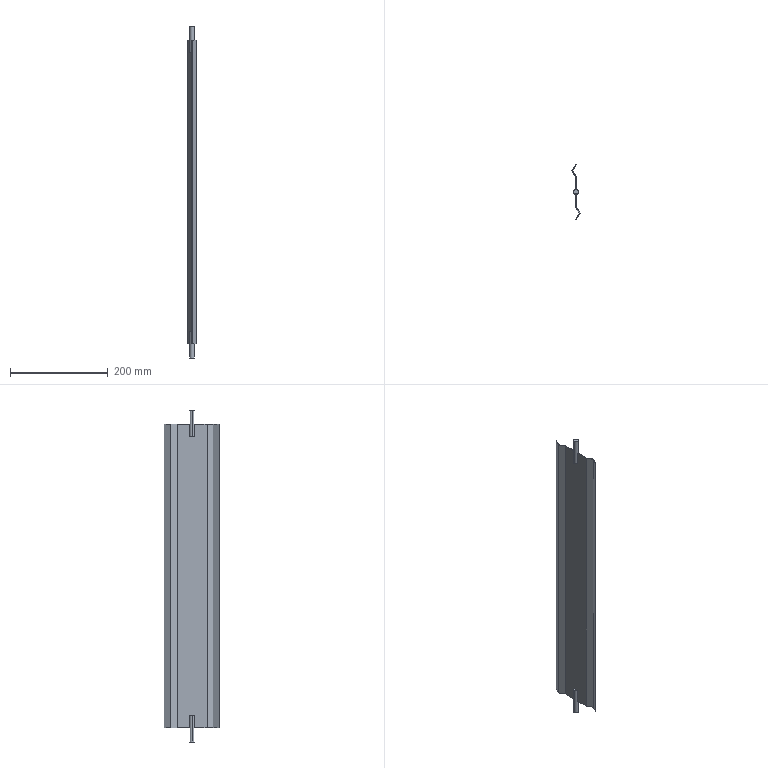Part | SolidWorks | features Extrusion 1, ICE 1, MirrorPattern 1 | 1 solid | 26 faces | box 16.5 x 113 x 678 mm | volume 119565 mm3 | plane 22 | cylinder 4 | commonest cylinder face diameters 10 x4
STEP:
#1=CARTESIAN_POINT('',(4.25,56.5,-284.));
#2=VERTEX_POINT('',#1);
#3=CARTESIAN_POINT('',(0.,61.443,-284.));
#4=VERTEX_POINT('',#3);
#5=CARTESIAN_POINT('',(-0.75,56.5,-284.));
#6=DIRECTION('',(0.,0.,1.));
#7=DIRECTION('',(1.,0.,0.));
#8=AXIS2_PLACEMENT_3D('',#5,#6,#7);
#9=CIRCLE('',#8,5.);
#10=EDGE_CURVE('',#2,#4,#9,.T.);
#11=ORIENTED_EDGE('',*,*,#10,.F.);
#12=CARTESIAN_POINT('',(4.25,56.5,-339.));
#13=VERTEX_POINT('',#12);
#14=CARTESIAN_POINT('',(4.25,56.5,-284.));
#15=DIRECTION('',(0.,0.,-1.));
#16=VECTOR('',#15,1000.);
#17=LINE('',#14,#16);
#18=EDGE_CURVE('',#2,#13,#17,.T.);
#19=ORIENTED_EDGE('',*,*,#18,.T.);
#20=CARTESIAN_POINT('',(-5.75,56.5,-339.));
#21=VERTEX_POINT('',#20);
#22=CARTESIAN_POINT('',(-0.75,56.5,-339.));
#23=DIRECTION('',(0.,0.,1.));
#24=DIRECTION('',(1.,0.,0.));
#25=AXIS2_PLACEMENT_3D('',#22,#23,#24);
#26=CIRCLE('',#25,5.);
#27=EDGE_CURVE('',#13,#21,#26,.T.);
#28=ORIENTED_EDGE('',*,*,#27,.T.);
#29=CARTESIAN_POINT('',(-5.75,56.5,-284.));
#30=VERTEX_POINT('',#29);
#31=CARTESIAN_POINT('',(-5.75,56.5,-284.));
#32=DIRECTION('',(0.,0.,-1.));
#33=VECTOR('',#32,1000.);
#34=LINE('',#31,#33);
#35=EDGE_CURVE('',#30,#21,#34,.T.);
#36=ORIENTED_EDGE('',*,*,#35,.F.);
#37=CARTESIAN_POINT('',(-1.5,61.443,-284.));
#38=VERTEX_POINT('',#37);
#39=CARTESIAN_POINT('',(-0.75,56.5,-284.));
#40=DIRECTION('',(0.,0.,1.));
#41=DIRECTION('',(1.,0.,0.));
#42=AXIS2_PLACEMENT_3D('',#39,#40,#41);
#43=CIRCLE('',#42,5.);
#44=EDGE_CURVE('',#38,#30,#43,.T.);
#45=ORIENTED_EDGE('',*,*,#44,.F.);
#46=CARTESIAN_POINT('',(-1.5,61.443,-310.));
#47=VERTEX_POINT('',#46);
#48=CARTESIAN_POINT('',(-1.5,61.443,-284.));
#49=DIRECTION('',(0.,0.,-1.));
#50=VECTOR('',#49,1000.);
#51=LINE('',#48,#50);
#52=EDGE_CURVE('',#38,#47,#51,.T.);
#53=ORIENTED_EDGE('',*,*,#52,.T.);
#54=CARTESIAN_POINT('',(0.,61.443,-310.));
#55=VERTEX_POINT('',#54);
#56=CARTESIAN_POINT('',(-0.75,56.5,-310.));
#57=DIRECTION('',(0.,0.,1.));
#58=DIRECTION('',(-1.,0.,0.));
#59=AXIS2_PLACEMENT_3D('',#56,#57,#58);
#60=CIRCLE('',#59,5.);
#61=EDGE_CURVE('',#55,#47,#60,.T.);
#62=ORIENTED_EDGE('',*,*,#61,.F.);
#63=CARTESIAN_POINT('',(0.,61.443,-284.));
#64=DIRECTION('',(0.,0.,1.));
#65=VECTOR('',#64,1000.);
#66=LINE('',#63,#65);
#67=EDGE_CURVE('',#55,#4,#66,.T.);
#68=ORIENTED_EDGE('',*,*,#67,.T.);
#69=EDGE_LOOP('',(#11,#19,#28,#36,#45,#53,#62,#68));
#70=FACE_OUTER_BOUND('',#69,.T.);
#71=CARTESIAN_POINT('',(-0.75,56.5,-284.));
#72=DIRECTION('',(0.,0.,-1.));
#73=DIRECTION('',(-1.,0.,0.));
#74=AXIS2_PLACEMENT_3D('',#71,#72,#73);
#75=CYLINDRICAL_SURFACE('',#74,5.);
#76=ADVANCED_FACE('',(#70),#75,.T.);
#77=CARTESIAN_POINT('',(-1.5,61.443,284.));
#78=VERTEX_POINT('',#77);
#79=CARTESIAN_POINT('',(-5.75,56.5,284.));
#80=VERTEX_POINT('',#79);
#81=CARTESIAN_POINT('',(-0.75,56.5,284.));
#82=DIRECTION('',(0.,0.,1.));
#83=DIRECTION('',(1.,0.,0.));
#84=AXIS2_PLACEMENT_3D('',#81,#82,#83);
#85=CIRCLE('',#84,5.);
#86=EDGE_CURVE('',#78,#80,#85,.T.);
#87=ORIENTED_EDGE('',*,*,#86,.T.);
#88=CARTESIAN_POINT('',(-5.75,56.5,339.));
#89=VERTEX_POINT('',#88);
#90=CARTESIAN_POINT('',(-5.75,56.5,284.));
#91=DIRECTION('',(0.,0.,1.));
#92=VECTOR('',#91,1000.);
#93=LINE('',#90,#92);
#94=EDGE_CURVE('',#80,#89,#93,.T.);
#95=ORIENTED_EDGE('',*,*,#94,.T.);
#96=CARTESIAN_POINT('',(4.25,56.5,339.));
#97=VERTEX_POINT('',#96);
#98=CARTESIAN_POINT('',(-0.75,56.5,339.));
#99=DIRECTION('',(0.,0.,1.));
#100=DIRECTION('',(1.,0.,0.));
#101=AXIS2_PLACEMENT_3D('',#98,#99,#100);
#102=CIRCLE('',#101,5.);
#103=EDGE_CURVE('',#97,#89,#102,.T.);
#104=ORIENTED_EDGE('',*,*,#103,.F.);
#105=CARTESIAN_POINT('',(4.25,56.5,284.));
#106=VERTEX_POINT('',#105);
#107=CARTESIAN_POINT('',(4.25,56.5,284.));
#108=DIRECTION('',(0.,0.,1.));
#109=VECTOR('',#108,1000.);
#110=LINE('',#107,#109);
#111=EDGE_CURVE('',#106,#97,#110,.T.);
#112=ORIENTED_EDGE('',*,*,#111,.F.);
#113=CARTESIAN_POINT('',(0.,61.443,284.));
#114=VERTEX_POINT('',#113);
#115=CARTESIAN_POINT('',(-0.75,56.5,284.));
#116=DIRECTION('',(0.,0.,1.));
#117=DIRECTION('',(1.,0.,0.));
#118=AXIS2_PLACEMENT_3D('',#115,#116,#117);
#119=CIRCLE('',#118,5.);
#120=EDGE_CURVE('',#106,#114,#119,.T.);
#121=ORIENTED_EDGE('',*,*,#120,.T.);
#122=CARTESIAN_POINT('',(0.,61.443,310.));
#123=VERTEX_POINT('',#122);
#124=CARTESIAN_POINT('',(0.,61.443,284.));
#125=DIRECTION('',(0.,0.,-1.));
#126=VECTOR('',#125,1000.);
#127=LINE('',#124,#126);
#128=EDGE_CURVE('',#123,#114,#127,.T.);
#129=ORIENTED_EDGE('',*,*,#128,.F.);
#130=CARTESIAN_POINT('',(-1.5,61.443,310.));
#131=VERTEX_POINT('',#130);
#132=CARTESIAN_POINT('',(-0.75,56.5,310.));
#133=DIRECTION('',(0.,0.,-1.));
#134=DIRECTION('',(-1.,0.,0.));
#135=AXIS2_PLACEMENT_3D('',#132,#133,#134);
#136=CIRCLE('',#135,5.);
#137=EDGE_CURVE('',#131,#123,#136,.T.);
#138=ORIENTED_EDGE('',*,*,#137,.F.);
#139=CARTESIAN_POINT('',(-1.5,61.443,284.));
#140=DIRECTION('',(0.,0.,1.));
#141=VECTOR('',#140,1000.);
#142=LINE('',#139,#141);
#143=EDGE_CURVE('',#78,#131,#142,.T.);
#144=ORIENTED_EDGE('',*,*,#143,.F.);
#145=EDGE_LOOP('',(#87,#95,#104,#112,#121,#129,#138,#144));
#146=FACE_OUTER_BOUND('',#145,.T.);
#147=CARTESIAN_POINT('',(-0.75,56.5,284.));
#148=DIRECTION('',(0.,0.,1.));
#149=DIRECTION('',(1.,0.,0.));
#150=AXIS2_PLACEMENT_3D('',#147,#148,#149);
#151=CYLINDRICAL_SURFACE('',#150,5.);
#152=ADVANCED_FACE('',(#146),#151,.T.);
#153=ORIENTED_EDGE('',*,*,#67,.F.);
#154=CARTESIAN_POINT('',(0.,87.421,-310.));
#155=VERTEX_POINT('',#154);
#156=CARTESIAN_POINT('',(0.,25.981,-310.));
#157=DIRECTION('',(0.,1.,0.));
#158=VECTOR('',#157,1000.);
#159=LINE('',#156,#158);
#160=EDGE_CURVE('',#55,#155,#159,.T.);
#161=ORIENTED_EDGE('',*,*,#160,.T.);
#162=CARTESIAN_POINT('',(0.,87.421,310.));
#163=VERTEX_POINT('',#162);
#164=CARTESIAN_POINT('',(0.,87.421,310.));
#165=DIRECTION('',(0.,0.,-1.));
#166=VECTOR('',#165,1000.);
#167=LINE('',#164,#166);
#168=EDGE_CURVE('',#163,#155,#167,.T.);
#169=ORIENTED_EDGE('',*,*,#168,.F.);
#170=CARTESIAN_POINT('',(0.,25.981,310.));
#171=DIRECTION('',(0.,1.,0.));
#172=VECTOR('',#171,1000.);
#173=LINE('',#170,#172);
#174=EDGE_CURVE('',#123,#163,#173,.T.);
#175=ORIENTED_EDGE('',*,*,#174,.F.);
#176=ORIENTED_EDGE('',*,*,#128,.T.);
#177=CARTESIAN_POINT('',(0.,51.557,284.));
#178=VERTEX_POINT('',#177);
#179=CARTESIAN_POINT('',(0.,25.981,284.));
#180=DIRECTION('',(0.,1.,0.));
#181=VECTOR('',#180,1000.);
#182=LINE('',#179,#181);
#183=EDGE_CURVE('',#178,#114,#182,.T.);
#184=ORIENTED_EDGE('',*,*,#183,.F.);
#185=CARTESIAN_POINT('',(0.,51.557,310.));
#186=VERTEX_POINT('',#185);
#187=CARTESIAN_POINT('',(0.,51.557,284.));
#188=DIRECTION('',(0.,0.,1.));
#189=VECTOR('',#188,1000.);
#190=LINE('',#187,#189);
#191=EDGE_CURVE('',#178,#186,#190,.T.);
#192=ORIENTED_EDGE('',*,*,#191,.T.);
#193=CARTESIAN_POINT('',(0.,25.981,310.));
#194=VERTEX_POINT('',#193);
#195=CARTESIAN_POINT('',(0.,25.981,310.));
#196=DIRECTION('',(0.,1.,0.));
#197=VECTOR('',#196,1000.);
#198=LINE('',#195,#197);
#199=EDGE_CURVE('',#194,#186,#198,.T.);
#200=ORIENTED_EDGE('',*,*,#199,.F.);
#201=CARTESIAN_POINT('',(0.,25.981,-310.));
#202=VERTEX_POINT('',#201);
#203=CARTESIAN_POINT('',(0.,25.981,310.));
#204=DIRECTION('',(0.,0.,-1.));
#205=VECTOR('',#204,1000.);
#206=LINE('',#203,#205);
#207=EDGE_CURVE('',#194,#202,#206,.T.);
#208=ORIENTED_EDGE('',*,*,#207,.T.);
#209=CARTESIAN_POINT('',(0.,51.557,-310.));
#210=VERTEX_POINT('',#209);
#211=CARTESIAN_POINT('',(0.,25.981,-310.));
#212=DIRECTION('',(0.,1.,0.));
#213=VECTOR('',#212,1000.);
#214=LINE('',#211,#213);
#215=EDGE_CURVE('',#202,#210,#214,.T.);
#216=ORIENTED_EDGE('',*,*,#215,.T.);
#217=CARTESIAN_POINT('',(0.,51.557,-284.));
#218=VERTEX_POINT('',#217);
#219=CARTESIAN_POINT('',(0.,51.557,-284.));
#220=DIRECTION('',(0.,0.,-1.));
#221=VECTOR('',#220,1000.);
#222=LINE('',#219,#221);
#223=EDGE_CURVE('',#218,#210,#222,.T.);
#224=ORIENTED_EDGE('',*,*,#223,.F.);
#225=CARTESIAN_POINT('',(0.,25.981,-284.));
#226=DIRECTION('',(0.,-1.,0.));
#227=VECTOR('',#226,1000.);
#228=LINE('',#225,#227);
#229=EDGE_CURVE('',#4,#218,#228,.T.);
#230=ORIENTED_EDGE('',*,*,#229,.F.);
#231=EDGE_LOOP('',(#153,#161,#169,#175,#176,#184,#192,#200,#208,#216,#224,#230));
#232=FACE_OUTER_BOUND('',#231,.T.);
#233=CARTESIAN_POINT('',(0.,25.981,310.));
#234=DIRECTION('',(-1.,0.,0.));
#235=DIRECTION('',(0.,-1.,0.));
#236=AXIS2_PLACEMENT_3D('',#233,#234,#235);
#237=PLANE('',#236);
#238=ADVANCED_FACE('',(#232),#237,.F.);
#239=CARTESIAN_POINT('',(-1.5,51.557,-310.));
#240=VERTEX_POINT('',#239);
#241=CARTESIAN_POINT('',(-1.5,51.557,-284.));
#242=VERTEX_POINT('',#241);
#243=CARTESIAN_POINT('',(-1.5,51.557,-284.));
#244=DIRECTION('',(0.,0.,1.));
#245=VECTOR('',#244,1000.);
#246=LINE('',#243,#245);
#247=EDGE_CURVE('',#240,#242,#246,.T.);
#248=ORIENTED_EDGE('',*,*,#247,.F.);
#249=CARTESIAN_POINT('',(-1.5,25.579,-310.));
#250=VERTEX_POINT('',#249);
#251=CARTESIAN_POINT('',(-1.5,25.579,-310.));
#252=DIRECTION('',(0.,-1.,0.));
#253=VECTOR('',#252,1000.);
#254=LINE('',#251,#253);
#255=EDGE_CURVE('',#240,#250,#254,.T.);
#256=ORIENTED_EDGE('',*,*,#255,.T.);
#257=CARTESIAN_POINT('',(-1.5,25.579,310.));
#258=VERTEX_POINT('',#257);
#259=CARTESIAN_POINT('',(-1.5,25.579,310.));
#260=DIRECTION('',(0.,0.,-1.));
#261=VECTOR('',#260,1000.);
#262=LINE('',#259,#261);
#263=EDGE_CURVE('',#258,#250,#262,.T.);
#264=ORIENTED_EDGE('',*,*,#263,.F.);
#265=CARTESIAN_POINT('',(-1.5,51.557,310.));
#266=VERTEX_POINT('',#265);
#267=CARTESIAN_POINT('',(-1.5,25.579,310.));
#268=DIRECTION('',(0.,-1.,0.));
#269=VECTOR('',#268,1000.);
#270=LINE('',#267,#269);
#271=EDGE_CURVE('',#266,#258,#270,.T.);
#272=ORIENTED_EDGE('',*,*,#271,.F.);
#273=CARTESIAN_POINT('',(-1.5,51.557,284.));
#274=VERTEX_POINT('',#273);
#275=CARTESIAN_POINT('',(-1.5,51.557,284.));
#276=DIRECTION('',(0.,0.,-1.));
#277=VECTOR('',#276,1000.);
#278=LINE('',#275,#277);
#279=EDGE_CURVE('',#266,#274,#278,.T.);
#280=ORIENTED_EDGE('',*,*,#279,.T.);
#281=CARTESIAN_POINT('',(-1.5,25.579,284.));
#282=DIRECTION('',(0.,-1.,0.));
#283=VECTOR('',#282,1000.);
#284=LINE('',#281,#283);
#285=EDGE_CURVE('',#78,#274,#284,.T.);
#286=ORIENTED_EDGE('',*,*,#285,.F.);
#287=ORIENTED_EDGE('',*,*,#143,.T.);
#288=CARTESIAN_POINT('',(-1.5,87.019,310.));
#289=VERTEX_POINT('',#288);
#290=CARTESIAN_POINT('',(-1.5,25.579,310.));
#291=DIRECTION('',(0.,-1.,0.));
#292=VECTOR('',#291,1000.);
#293=LINE('',#290,#292);
#294=EDGE_CURVE('',#289,#131,#293,.T.);
#295=ORIENTED_EDGE('',*,*,#294,.F.);
#296=CARTESIAN_POINT('',(-1.5,87.019,-310.));
#297=VERTEX_POINT('',#296);
#298=CARTESIAN_POINT('',(-1.5,87.019,310.));
#299=DIRECTION('',(0.,0.,-1.));
#300=VECTOR('',#299,1000.);
#301=LINE('',#298,#300);
#302=EDGE_CURVE('',#289,#297,#301,.T.);
#303=ORIENTED_EDGE('',*,*,#302,.T.);
#304=CARTESIAN_POINT('',(-1.5,25.579,-310.));
#305=DIRECTION('',(0.,-1.,0.));
#306=VECTOR('',#305,1000.);
#307=LINE('',#304,#306);
#308=EDGE_CURVE('',#297,#47,#307,.T.);
#309=ORIENTED_EDGE('',*,*,#308,.T.);
#310=ORIENTED_EDGE('',*,*,#52,.F.);
#311=CARTESIAN_POINT('',(-1.5,25.579,-284.));
#312=DIRECTION('',(0.,1.,0.));
#313=VECTOR('',#312,1000.);
#314=LINE('',#311,#313);
#315=EDGE_CURVE('',#242,#38,#314,.T.);
#316=ORIENTED_EDGE('',*,*,#315,.F.);
#317=EDGE_LOOP('',(#248,#256,#264,#272,#280,#286,#287,#295,#303,#309,#310,#316));
#318=FACE_OUTER_BOUND('',#317,.T.);
#319=CARTESIAN_POINT('',(-1.5,25.579,310.));
#320=DIRECTION('',(1.,0.,0.));
#321=DIRECTION('',(0.,1.,0.));
#322=AXIS2_PLACEMENT_3D('',#319,#320,#321);
#323=PLANE('',#322);
#324=ADVANCED_FACE('',(#318),#323,.F.);
#325=ORIENTED_EDGE('',*,*,#255,.F.);
#326=CARTESIAN_POINT('',(-0.75,56.5,-310.));
#327=DIRECTION('',(0.,0.,1.));
#328=DIRECTION('',(-1.,0.,0.));
#329=AXIS2_PLACEMENT_3D('',#326,#327,#328);
#330=CIRCLE('',#329,5.);
#331=EDGE_CURVE('',#240,#210,#330,.T.);
#332=ORIENTED_EDGE('',*,*,#331,.T.);
#333=ORIENTED_EDGE('',*,*,#215,.F.);
#334=CARTESIAN_POINT('',(7.5,12.99,-310.));
#335=VERTEX_POINT('',#334);
#336=CARTESIAN_POINT('',(7.5,12.99,-310.));
#337=DIRECTION('',(-0.5,0.866,0.));
#338=VECTOR('',#337,1000.);
#339=LINE('',#336,#338);
#340=EDGE_CURVE('',#335,#202,#339,.T.);
#341=ORIENTED_EDGE('',*,*,#340,.F.);
#342=CARTESIAN_POINT('',(0.,0.,-310.));
#343=VERTEX_POINT('',#342);
#344=CARTESIAN_POINT('',(0.,0.,-310.));
#345=DIRECTION('',(0.5,0.866,0.));
#346=VECTOR('',#345,1000.);
#347=LINE('',#344,#346);
#348=EDGE_CURVE('',#343,#335,#347,.T.);
#349=ORIENTED_EDGE('',*,*,#348,.F.);
#350=CARTESIAN_POINT('',(-1.299,0.75,-310.));
#351=VERTEX_POINT('',#350);
#352=CARTESIAN_POINT('',(0.,0.,-310.));
#353=DIRECTION('',(0.866,-0.5,0.));
#354=VECTOR('',#353,1000.);
#355=LINE('',#352,#354);
#356=EDGE_CURVE('',#351,#343,#355,.T.);
#357=ORIENTED_EDGE('',*,*,#356,.F.);
#358=CARTESIAN_POINT('',(5.768,12.99,-310.));
#359=VERTEX_POINT('',#358);
#360=CARTESIAN_POINT('',(-1.299,0.75,-310.));
#361=DIRECTION('',(-0.5,-0.866,0.));
#362=VECTOR('',#361,1000.);
#363=LINE('',#360,#362);
#364=EDGE_CURVE('',#359,#351,#363,.T.);
#365=ORIENTED_EDGE('',*,*,#364,.F.);
#366=CARTESIAN_POINT('',(5.768,12.99,-310.));
#367=DIRECTION('',(0.5,-0.866,0.));
#368=VECTOR('',#367,1000.);
#369=LINE('',#366,#368);
#370=EDGE_CURVE('',#250,#359,#369,.T.);
#371=ORIENTED_EDGE('',*,*,#370,.F.);
#372=EDGE_LOOP('',(#325,#332,#333,#341,#349,#357,#365,#371));
#373=FACE_OUTER_BOUND('',#372,.T.);
#374=CARTESIAN_POINT('',(0.,0.,-310.));
#375=DIRECTION('',(0.,0.,-1.));
#376=DIRECTION('',(-1.,0.,0.));
#377=AXIS2_PLACEMENT_3D('',#374,#375,#376);
#378=PLANE('',#377);
#379=ADVANCED_FACE('',(#373),#378,.T.);
#380=ORIENTED_EDGE('',*,*,#294,.T.);
#381=ORIENTED_EDGE('',*,*,#137,.T.);
#382=ORIENTED_EDGE('',*,*,#174,.T.);
#383=CARTESIAN_POINT('',(-7.268,100.01,310.));
#384=VERTEX_POINT('',#383);
#385=CARTESIAN_POINT('',(0.,87.421,310.));
#386=DIRECTION('',(-0.5,0.866,0.));
#387=VECTOR('',#386,1000.);
#388=LINE('',#385,#387);
#389=EDGE_CURVE('',#163,#384,#388,.T.);
#390=ORIENTED_EDGE('',*,*,#389,.T.);
#391=CARTESIAN_POINT('',(-0.201,112.25,310.));
#392=VERTEX_POINT('',#391);
#393=CARTESIAN_POINT('',(-7.268,100.01,310.));
#394=DIRECTION('',(0.5,0.866,0.));
#395=VECTOR('',#394,1000.);
#396=LINE('',#393,#395);
#397=EDGE_CURVE('',#384,#392,#396,.T.);
#398=ORIENTED_EDGE('',*,*,#397,.T.);
#399=CARTESIAN_POINT('',(-1.5,113.,310.));
#400=VERTEX_POINT('',#399);
#401=CARTESIAN_POINT('',(-0.201,112.25,310.));
#402=DIRECTION('',(-0.866,0.5,0.));
#403=VECTOR('',#402,1000.);
#404=LINE('',#401,#403);
#405=EDGE_CURVE('',#392,#400,#404,.T.);
#406=ORIENTED_EDGE('',*,*,#405,.T.);
#407=CARTESIAN_POINT('',(-9.,100.01,310.));
#408=VERTEX_POINT('',#407);
#409=CARTESIAN_POINT('',(-9.,100.01,310.));
#410=DIRECTION('',(-0.5,-0.866,0.));
#411=VECTOR('',#410,1000.);
#412=LINE('',#409,#411);
#413=EDGE_CURVE('',#400,#408,#412,.T.);
#414=ORIENTED_EDGE('',*,*,#413,.T.);
#415=CARTESIAN_POINT('',(-1.5,87.019,310.));
#416=DIRECTION('',(0.5,-0.866,0.));
#417=VECTOR('',#416,1000.);
#418=LINE('',#415,#417);
#419=EDGE_CURVE('',#408,#289,#418,.T.);
#420=ORIENTED_EDGE('',*,*,#419,.T.);
#421=EDGE_LOOP('',(#380,#381,#382,#390,#398,#406,#414,#420));
#422=FACE_OUTER_BOUND('',#421,.T.);
#423=CARTESIAN_POINT('',(0.,0.,310.));
#424=DIRECTION('',(0.,0.,-1.));
#425=DIRECTION('',(-1.,0.,0.));
#426=AXIS2_PLACEMENT_3D('',#423,#424,#425);
#427=PLANE('',#426);
#428=ADVANCED_FACE('',(#422),#427,.F.);
#429=ORIENTED_EDGE('',*,*,#356,.T.);
#430=CARTESIAN_POINT('',(0.,0.,310.));
#431=VERTEX_POINT('',#430);
#432=CARTESIAN_POINT('',(0.,0.,310.));
#433=DIRECTION('',(0.,0.,-1.));
#434=VECTOR('',#433,1000.);
#435=LINE('',#432,#434);
#436=EDGE_CURVE('',#431,#343,#435,.T.);
#437=ORIENTED_EDGE('',*,*,#436,.F.);
#438=CARTESIAN_POINT('',(-1.299,0.75,310.));
#439=VERTEX_POINT('',#438);
#440=CARTESIAN_POINT('',(0.,0.,310.));
#441=DIRECTION('',(0.866,-0.5,0.));
#442=VECTOR('',#441,1000.);
#443=LINE('',#440,#442);
#444=EDGE_CURVE('',#439,#431,#443,.T.);
#445=ORIENTED_EDGE('',*,*,#444,.F.);
#446=CARTESIAN_POINT('',(-1.299,0.75,310.));
#447=DIRECTION('',(0.,0.,-1.));
#448=VECTOR('',#447,1000.);
#449=LINE('',#446,#448);
#450=EDGE_CURVE('',#439,#351,#449,.T.);
#451=ORIENTED_EDGE('',*,*,#450,.T.);
#452=EDGE_LOOP('',(#429,#437,#445,#451));
#453=FACE_OUTER_BOUND('',#452,.T.);
#454=CARTESIAN_POINT('',(0.,0.,310.));
#455=DIRECTION('',(0.5,0.866,0.));
#456=DIRECTION('',(-0.866,0.5,0.));
#457=AXIS2_PLACEMENT_3D('',#454,#455,#456);
#458=PLANE('',#457);
#459=ADVANCED_FACE('',(#453),#458,.F.);
#460=ORIENTED_EDGE('',*,*,#348,.T.);
#461=CARTESIAN_POINT('',(7.5,12.99,310.));
#462=VERTEX_POINT('',#461);
#463=CARTESIAN_POINT('',(7.5,12.99,310.));
#464=DIRECTION('',(0.,0.,-1.));
#465=VECTOR('',#464,1000.);
#466=LINE('',#463,#465);
#467=EDGE_CURVE('',#462,#335,#466,.T.);
#468=ORIENTED_EDGE('',*,*,#467,.F.);
#469=CARTESIAN_POINT('',(0.,0.,310.));
#470=DIRECTION('',(0.5,0.866,0.));
#471=VECTOR('',#470,1000.);
#472=LINE('',#469,#471);
#473=EDGE_CURVE('',#431,#462,#472,.T.);
#474=ORIENTED_EDGE('',*,*,#473,.F.);
#475=ORIENTED_EDGE('',*,*,#436,.T.);
#476=EDGE_LOOP('',(#460,#468,#474,#475));
#477=FACE_OUTER_BOUND('',#476,.T.);
#478=CARTESIAN_POINT('',(0.,0.,310.));
#479=DIRECTION('',(-0.866,0.5,0.));
#480=DIRECTION('',(-0.5,-0.866,0.));
#481=AXIS2_PLACEMENT_3D('',#478,#479,#480);
#482=PLANE('',#481);
#483=ADVANCED_FACE('',(#477),#482,.F.);
#484=ORIENTED_EDGE('',*,*,#340,.T.);
#485=ORIENTED_EDGE('',*,*,#207,.F.);
#486=CARTESIAN_POINT('',(7.5,12.99,310.));
#487=DIRECTION('',(-0.5,0.866,0.));
#488=VECTOR('',#487,1000.);
#489=LINE('',#486,#488);
#490=EDGE_CURVE('',#462,#194,#489,.T.);
#491=ORIENTED_EDGE('',*,*,#490,.F.);
#492=ORIENTED_EDGE('',*,*,#467,.T.);
#493=EDGE_LOOP('',(#484,#485,#491,#492));
#494=FACE_OUTER_BOUND('',#493,.T.);
#495=CARTESIAN_POINT('',(7.5,12.99,310.));
#496=DIRECTION('',(-0.866,-0.5,0.));
#497=DIRECTION('',(0.5,-0.866,0.));
#498=AXIS2_PLACEMENT_3D('',#495,#496,#497);
#499=PLANE('',#498);
#500=ADVANCED_FACE('',(#494),#499,.F.);
#501=CARTESIAN_POINT('',(-7.268,100.01,-310.));
#502=VERTEX_POINT('',#501);
#503=CARTESIAN_POINT('',(0.,87.421,-310.));
#504=DIRECTION('',(-0.5,0.866,0.));
#505=VECTOR('',#504,1000.);
#506=LINE('',#503,#505);
#507=EDGE_CURVE('',#155,#502,#506,.T.);
#508=ORIENTED_EDGE('',*,*,#507,.T.);
#509=CARTESIAN_POINT('',(-7.268,100.01,310.));
#510=DIRECTION('',(0.,0.,-1.));
#511=VECTOR('',#510,1000.);
#512=LINE('',#509,#511);
#513=EDGE_CURVE('',#384,#502,#512,.T.);
#514=ORIENTED_EDGE('',*,*,#513,.F.);
#515=ORIENTED_EDGE('',*,*,#389,.F.);
#516=ORIENTED_EDGE('',*,*,#168,.T.);
#517=EDGE_LOOP('',(#508,#514,#515,#516));
#518=FACE_OUTER_BOUND('',#517,.T.);
#519=CARTESIAN_POINT('',(0.,87.421,310.));
#520=DIRECTION('',(-0.866,-0.5,0.));
#521=DIRECTION('',(0.5,-0.866,0.));
#522=AXIS2_PLACEMENT_3D('',#519,#520,#521);
#523=PLANE('',#522);
#524=ADVANCED_FACE('',(#518),#523,.F.);
#525=CARTESIAN_POINT('',(-0.201,112.25,-310.));
#526=VERTEX_POINT('',#525);
#527=CARTESIAN_POINT('',(-7.268,100.01,-310.));
#528=DIRECTION('',(0.5,0.866,0.));
#529=VECTOR('',#528,1000.);
#530=LINE('',#527,#529);
#531=EDGE_CURVE('',#502,#526,#530,.T.);
#532=ORIENTED_EDGE('',*,*,#531,.T.);
#533=CARTESIAN_POINT('',(-0.201,112.25,310.));
#534=DIRECTION('',(0.,0.,-1.));
#535=VECTOR('',#534,1000.);
#536=LINE('',#533,#535);
#537=EDGE_CURVE('',#392,#526,#536,.T.);
#538=ORIENTED_EDGE('',*,*,#537,.F.);
#539=ORIENTED_EDGE('',*,*,#397,.F.);
#540=ORIENTED_EDGE('',*,*,#513,.T.);
#541=EDGE_LOOP('',(#532,#538,#539,#540));
#542=FACE_OUTER_BOUND('',#541,.T.);
#543=CARTESIAN_POINT('',(-7.268,100.01,310.));
#544=DIRECTION('',(-0.866,0.5,0.));
#545=DIRECTION('',(-0.5,-0.866,0.));
#546=AXIS2_PLACEMENT_3D('',#543,#544,#545);
#547=PLANE('',#546);
#548=ADVANCED_FACE('',(#542),#547,.F.);
#549=CARTESIAN_POINT('',(-1.5,113.,-310.));
#550=VERTEX_POINT('',#549);
#551=CARTESIAN_POINT('',(-0.201,112.25,-310.));
#552=DIRECTION('',(-0.866,0.5,0.));
#553=VECTOR('',#552,1000.);
#554=LINE('',#551,#553);
#555=EDGE_CURVE('',#526,#550,#554,.T.);
#556=ORIENTED_EDGE('',*,*,#555,.T.);
#557=CARTESIAN_POINT('',(-1.5,113.,310.));
#558=DIRECTION('',(0.,0.,-1.));
#559=VECTOR('',#558,1000.);
#560=LINE('',#557,#559);
#561=EDGE_CURVE('',#400,#550,#560,.T.);
#562=ORIENTED_EDGE('',*,*,#561,.F.);
#563=ORIENTED_EDGE('',*,*,#405,.F.);
#564=ORIENTED_EDGE('',*,*,#537,.T.);
#565=EDGE_LOOP('',(#556,#562,#563,#564));
#566=FACE_OUTER_BOUND('',#565,.T.);
#567=CARTESIAN_POINT('',(-0.201,112.25,310.));
#568=DIRECTION('',(-0.5,-0.866,0.));
#569=DIRECTION('',(0.866,-0.5,0.));
#570=AXIS2_PLACEMENT_3D('',#567,#568,#569);
#571=PLANE('',#570);
#572=ADVANCED_FACE('',(#566),#571,.F.);
#573=CARTESIAN_POINT('',(-9.,100.01,-310.));
#574=VERTEX_POINT('',#573);
#575=CARTESIAN_POINT('',(-9.,100.01,-310.));
#576=DIRECTION('',(-0.5,-0.866,0.));
#577=VECTOR('',#576,1000.);
#578=LINE('',#575,#577);
#579=EDGE_CURVE('',#550,#574,#578,.T.);
#580=ORIENTED_EDGE('',*,*,#579,.T.);
#581=CARTESIAN_POINT('',(-9.,100.01,310.));
#582=DIRECTION('',(0.,0.,-1.));
#583=VECTOR('',#582,1000.);
#584=LINE('',#581,#583);
#585=EDGE_CURVE('',#408,#574,#584,.T.);
#586=ORIENTED_EDGE('',*,*,#585,.F.);
#587=ORIENTED_EDGE('',*,*,#413,.F.);
#588=ORIENTED_EDGE('',*,*,#561,.T.);
#589=EDGE_LOOP('',(#580,#586,#587,#588));
#590=FACE_OUTER_BOUND('',#589,.T.);
#591=CARTESIAN_POINT('',(-9.,100.01,310.));
#592=DIRECTION('',(0.866,-0.5,0.));
#593=DIRECTION('',(0.5,0.866,0.));
#594=AXIS2_PLACEMENT_3D('',#591,#592,#593);
#595=PLANE('',#594);
#596=ADVANCED_FACE('',(#590),#595,.F.);
#597=CARTESIAN_POINT('',(-1.5,87.019,-310.));
#598=DIRECTION('',(0.5,-0.866,0.));
#599=VECTOR('',#598,1000.);
#600=LINE('',#597,#599);
#601=EDGE_CURVE('',#574,#297,#600,.T.);
#602=ORIENTED_EDGE('',*,*,#601,.T.);
#603=ORIENTED_EDGE('',*,*,#302,.F.);
#604=ORIENTED_EDGE('',*,*,#419,.F.);
#605=ORIENTED_EDGE('',*,*,#585,.T.);
#606=EDGE_LOOP('',(#602,#603,#604,#605));
#607=FACE_OUTER_BOUND('',#606,.T.);
#608=CARTESIAN_POINT('',(-1.5,87.019,310.));
#609=DIRECTION('',(0.866,0.5,0.));
#610=DIRECTION('',(-0.5,0.866,0.));
#611=AXIS2_PLACEMENT_3D('',#608,#609,#610);
#612=PLANE('',#611);
#613=ADVANCED_FACE('',(#607),#612,.F.);
#614=ORIENTED_EDGE('',*,*,#370,.T.);
#615=CARTESIAN_POINT('',(5.768,12.99,310.));
#616=VERTEX_POINT('',#615);
#617=CARTESIAN_POINT('',(5.768,12.99,310.));
#618=DIRECTION('',(0.,0.,-1.));
#619=VECTOR('',#618,1000.);
#620=LINE('',#617,#619);
#621=EDGE_CURVE('',#616,#359,#620,.T.);
#622=ORIENTED_EDGE('',*,*,#621,.F.);
#623=CARTESIAN_POINT('',(5.768,12.99,310.));
#624=DIRECTION('',(0.5,-0.866,0.));
#625=VECTOR('',#624,1000.);
#626=LINE('',#623,#625);
#627=EDGE_CURVE('',#258,#616,#626,.T.);
#628=ORIENTED_EDGE('',*,*,#627,.F.);
#629=ORIENTED_EDGE('',*,*,#263,.T.);
#630=EDGE_LOOP('',(#614,#622,#628,#629));
#631=FACE_OUTER_BOUND('',#630,.T.);
#632=CARTESIAN_POINT('',(5.768,12.99,310.));
#633=DIRECTION('',(0.866,0.5,0.));
#634=DIRECTION('',(-0.5,0.866,0.));
#635=AXIS2_PLACEMENT_3D('',#632,#633,#634);
#636=PLANE('',#635);
#637=ADVANCED_FACE('',(#631),#636,.F.);
#638=ORIENTED_EDGE('',*,*,#364,.T.);
#639=ORIENTED_EDGE('',*,*,#450,.F.);
#640=CARTESIAN_POINT('',(-1.299,0.75,310.));
#641=DIRECTION('',(-0.5,-0.866,0.));
#642=VECTOR('',#641,1000.);
#643=LINE('',#640,#642);
#644=EDGE_CURVE('',#616,#439,#643,.T.);
#645=ORIENTED_EDGE('',*,*,#644,.F.);
#646=ORIENTED_EDGE('',*,*,#621,.T.);
#647=EDGE_LOOP('',(#638,#639,#645,#646));
#648=FACE_OUTER_BOUND('',#647,.T.);
#649=CARTESIAN_POINT('',(-1.299,0.75,310.));
#650=DIRECTION('',(0.866,-0.5,0.));
#651=DIRECTION('',(0.5,0.866,0.));
#652=AXIS2_PLACEMENT_3D('',#649,#650,#651);
#653=PLANE('',#652);
#654=ADVANCED_FACE('',(#648),#653,.F.);
#655=ORIENTED_EDGE('',*,*,#199,.T.);
#656=CARTESIAN_POINT('',(-0.75,56.5,310.));
#657=DIRECTION('',(0.,0.,-1.));
#658=DIRECTION('',(-1.,0.,0.));
#659=AXIS2_PLACEMENT_3D('',#656,#657,#658);
#660=CIRCLE('',#659,5.);
#661=EDGE_CURVE('',#186,#266,#660,.T.);
#662=ORIENTED_EDGE('',*,*,#661,.T.);
#663=ORIENTED_EDGE('',*,*,#271,.T.);
#664=ORIENTED_EDGE('',*,*,#627,.T.);
#665=ORIENTED_EDGE('',*,*,#644,.T.);
#666=ORIENTED_EDGE('',*,*,#444,.T.);
#667=ORIENTED_EDGE('',*,*,#473,.T.);
#668=ORIENTED_EDGE('',*,*,#490,.T.);
#669=EDGE_LOOP('',(#655,#662,#663,#664,#665,#666,#667,#668));
#670=FACE_OUTER_BOUND('',#669,.T.);
#671=CARTESIAN_POINT('',(0.,0.,310.));
#672=DIRECTION('',(0.,0.,-1.));
#673=DIRECTION('',(-1.,0.,0.));
#674=AXIS2_PLACEMENT_3D('',#671,#672,#673);
#675=PLANE('',#674);
#676=ADVANCED_FACE('',(#670),#675,.F.);
#677=ORIENTED_EDGE('',*,*,#160,.F.);
#678=ORIENTED_EDGE('',*,*,#61,.T.);
#679=ORIENTED_EDGE('',*,*,#308,.F.);
#680=ORIENTED_EDGE('',*,*,#601,.F.);
#681=ORIENTED_EDGE('',*,*,#579,.F.);
#682=ORIENTED_EDGE('',*,*,#555,.F.);
#683=ORIENTED_EDGE('',*,*,#531,.F.);
#684=ORIENTED_EDGE('',*,*,#507,.F.);
#685=EDGE_LOOP('',(#677,#678,#679,#680,#681,#682,#683,#684));
#686=FACE_OUTER_BOUND('',#685,.T.);
#687=CARTESIAN_POINT('',(0.,0.,-310.));
#688=DIRECTION('',(0.,0.,-1.));
#689=DIRECTION('',(-1.,0.,0.));
#690=AXIS2_PLACEMENT_3D('',#687,#688,#689);
#691=PLANE('',#690);
#692=ADVANCED_FACE('',(#686),#691,.T.);
#693=CARTESIAN_POINT('',(-0.75,56.5,284.));
#694=DIRECTION('',(0.,0.,1.));
#695=DIRECTION('',(1.,0.,0.));
#696=AXIS2_PLACEMENT_3D('',#693,#694,#695);
#697=CIRCLE('',#696,5.);
#698=EDGE_CURVE('',#178,#106,#697,.T.);
#699=ORIENTED_EDGE('',*,*,#698,.F.);
#700=ORIENTED_EDGE('',*,*,#183,.T.);
#701=ORIENTED_EDGE('',*,*,#120,.F.);
#702=EDGE_LOOP('',(#699,#700,#701));
#703=FACE_OUTER_BOUND('',#702,.T.);
#704=CARTESIAN_POINT('',(-0.75,56.5,284.));
#705=DIRECTION('',(0.,0.,1.));
#706=DIRECTION('',(1.,0.,0.));
#707=AXIS2_PLACEMENT_3D('',#704,#705,#706);
#708=PLANE('',#707);
#709=ADVANCED_FACE('',(#703),#708,.F.);
#710=ORIENTED_EDGE('',*,*,#86,.F.);
#711=ORIENTED_EDGE('',*,*,#285,.T.);
#712=CARTESIAN_POINT('',(-0.75,56.5,284.));
#713=DIRECTION('',(0.,0.,1.));
#714=DIRECTION('',(1.,0.,0.));
#715=AXIS2_PLACEMENT_3D('',#712,#713,#714);
#716=CIRCLE('',#715,5.);
#717=EDGE_CURVE('',#80,#274,#716,.T.);
#718=ORIENTED_EDGE('',*,*,#717,.F.);
#719=EDGE_LOOP('',(#710,#711,#718));
#720=FACE_OUTER_BOUND('',#719,.T.);
#721=CARTESIAN_POINT('',(-0.75,56.5,284.));
#722=DIRECTION('',(0.,0.,1.));
#723=DIRECTION('',(1.,0.,0.));
#724=AXIS2_PLACEMENT_3D('',#721,#722,#723);
#725=PLANE('',#724);
#726=ADVANCED_FACE('',(#720),#725,.F.);
#727=ORIENTED_EDGE('',*,*,#94,.F.);
#728=ORIENTED_EDGE('',*,*,#717,.T.);
#729=ORIENTED_EDGE('',*,*,#279,.F.);
#730=ORIENTED_EDGE('',*,*,#661,.F.);
#731=ORIENTED_EDGE('',*,*,#191,.F.);
#732=ORIENTED_EDGE('',*,*,#698,.T.);
#733=ORIENTED_EDGE('',*,*,#111,.T.);
#734=CARTESIAN_POINT('',(-0.75,56.5,339.));
#735=DIRECTION('',(0.,0.,1.));
#736=DIRECTION('',(1.,0.,0.));
#737=AXIS2_PLACEMENT_3D('',#734,#735,#736);
#738=CIRCLE('',#737,5.);
#739=EDGE_CURVE('',#89,#97,#738,.T.);
#740=ORIENTED_EDGE('',*,*,#739,.F.);
#741=EDGE_LOOP('',(#727,#728,#729,#730,#731,#732,#733,#740));
#742=FACE_OUTER_BOUND('',#741,.T.);
#743=CARTESIAN_POINT('',(-0.75,56.5,284.));
#744=DIRECTION('',(0.,0.,1.));
#745=DIRECTION('',(1.,0.,0.));
#746=AXIS2_PLACEMENT_3D('',#743,#744,#745);
#747=CYLINDRICAL_SURFACE('',#746,5.);
#748=ADVANCED_FACE('',(#742),#747,.T.);
#749=ORIENTED_EDGE('',*,*,#103,.T.);
#750=ORIENTED_EDGE('',*,*,#739,.T.);
#751=EDGE_LOOP('',(#749,#750));
#752=FACE_OUTER_BOUND('',#751,.T.);
#753=CARTESIAN_POINT('',(-0.75,56.5,339.));
#754=DIRECTION('',(0.,0.,1.));
#755=DIRECTION('',(1.,0.,0.));
#756=AXIS2_PLACEMENT_3D('',#753,#754,#755);
#757=PLANE('',#756);
#758=ADVANCED_FACE('',(#752),#757,.T.);
#759=CARTESIAN_POINT('',(-0.75,56.5,-284.));
#760=DIRECTION('',(0.,0.,1.));
#761=DIRECTION('',(1.,0.,0.));
#762=AXIS2_PLACEMENT_3D('',#759,#760,#761);
#763=CIRCLE('',#762,5.);
#764=EDGE_CURVE('',#218,#2,#763,.T.);
#765=ORIENTED_EDGE('',*,*,#764,.T.);
#766=ORIENTED_EDGE('',*,*,#10,.T.);
#767=ORIENTED_EDGE('',*,*,#229,.T.);
#768=EDGE_LOOP('',(#765,#766,#767));
#769=FACE_OUTER_BOUND('',#768,.T.);
#770=CARTESIAN_POINT('',(-0.75,56.5,-284.));
#771=DIRECTION('',(0.,0.,-1.));
#772=DIRECTION('',(1.,0.,0.));
#773=AXIS2_PLACEMENT_3D('',#770,#771,#772);
#774=PLANE('',#773);
#775=ADVANCED_FACE('',(#769),#774,.F.);
#776=ORIENTED_EDGE('',*,*,#44,.T.);
#777=CARTESIAN_POINT('',(-0.75,56.5,-284.));
#778=DIRECTION('',(0.,0.,1.));
#779=DIRECTION('',(1.,0.,0.));
#780=AXIS2_PLACEMENT_3D('',#777,#778,#779);
#781=CIRCLE('',#780,5.);
#782=EDGE_CURVE('',#30,#242,#781,.T.);
#783=ORIENTED_EDGE('',*,*,#782,.T.);
#784=ORIENTED_EDGE('',*,*,#315,.T.);
#785=EDGE_LOOP('',(#776,#783,#784));
#786=FACE_OUTER_BOUND('',#785,.T.);
#787=CARTESIAN_POINT('',(-0.75,56.5,-284.));
#788=DIRECTION('',(0.,0.,-1.));
#789=DIRECTION('',(1.,0.,0.));
#790=AXIS2_PLACEMENT_3D('',#787,#788,#789);
#791=PLANE('',#790);
#792=ADVANCED_FACE('',(#786),#791,.F.);
#793=ORIENTED_EDGE('',*,*,#18,.F.);
#794=ORIENTED_EDGE('',*,*,#764,.F.);
#795=ORIENTED_EDGE('',*,*,#223,.T.);
#796=ORIENTED_EDGE('',*,*,#331,.F.);
#797=ORIENTED_EDGE('',*,*,#247,.T.);
#798=ORIENTED_EDGE('',*,*,#782,.F.);
#799=ORIENTED_EDGE('',*,*,#35,.T.);
#800=CARTESIAN_POINT('',(-0.75,56.5,-339.));
#801=DIRECTION('',(0.,0.,1.));
#802=DIRECTION('',(1.,0.,0.));
#803=AXIS2_PLACEMENT_3D('',#800,#801,#802);
#804=CIRCLE('',#803,5.);
#805=EDGE_CURVE('',#21,#13,#804,.T.);
#806=ORIENTED_EDGE('',*,*,#805,.T.);
#807=EDGE_LOOP('',(#793,#794,#795,#796,#797,#798,#799,#806));
#808=FACE_OUTER_BOUND('',#807,.T.);
#809=CARTESIAN_POINT('',(-0.75,56.5,-284.));
#810=DIRECTION('',(0.,0.,-1.));
#811=DIRECTION('',(-1.,0.,0.));
#812=AXIS2_PLACEMENT_3D('',#809,#810,#811);
#813=CYLINDRICAL_SURFACE('',#812,5.);
#814=ADVANCED_FACE('',(#808),#813,.T.);
#815=ORIENTED_EDGE('',*,*,#805,.F.);
#816=ORIENTED_EDGE('',*,*,#27,.F.);
#817=EDGE_LOOP('',(#815,#816));
#818=FACE_OUTER_BOUND('',#817,.T.);
#819=CARTESIAN_POINT('',(-0.75,56.5,-339.));
#820=DIRECTION('',(0.,0.,-1.));
#821=DIRECTION('',(1.,0.,0.));
#822=AXIS2_PLACEMENT_3D('',#819,#820,#821);
#823=PLANE('',#822);
#824=ADVANCED_FACE('',(#818),#823,.T.);
#825=CLOSED_SHELL('',(#76,#152,#238,#324,#379,#428,#459,#483,#500,#524,#548,#572,#596,#613,#637,#654,#676,#692,#709,#726,#748,#758,#775,#792,#814,#824));
#826=MANIFOLD_SOLID_BREP('',#825);
#827=CARTESIAN_POINT('',(0.,0.,0.));
#828=DIRECTION('',(0.,0.,1.));
#829=DIRECTION('',(1.,0.,0.));
#830=AXIS2_PLACEMENT_3D('',#827,#828,#829);
#831=(LENGTH_UNIT()NAMED_UNIT(*)SI_UNIT(.MILLI.,.METRE.));
#832=UNCERTAINTY_MEASURE_WITH_UNIT(LENGTH_MEASURE(0.00001),#831,'','');
#833=(NAMED_UNIT(*)PLANE_ANGLE_UNIT()SI_UNIT($,.RADIAN.));
#834=(NAMED_UNIT(*)SI_UNIT($,.STERADIAN.)SOLID_ANGLE_UNIT());
#835=(GEOMETRIC_REPRESENTATION_CONTEXT(3)GLOBAL_UNCERTAINTY_ASSIGNED_CONTEXT((#832))GLOBAL_UNIT_ASSIGNED_CONTEXT((#831,#833,#834))REPRESENTATION_CONTEXT('',''));
#836=ADVANCED_BREP_SHAPE_REPRESENTATION('',(#826,#830),#835);